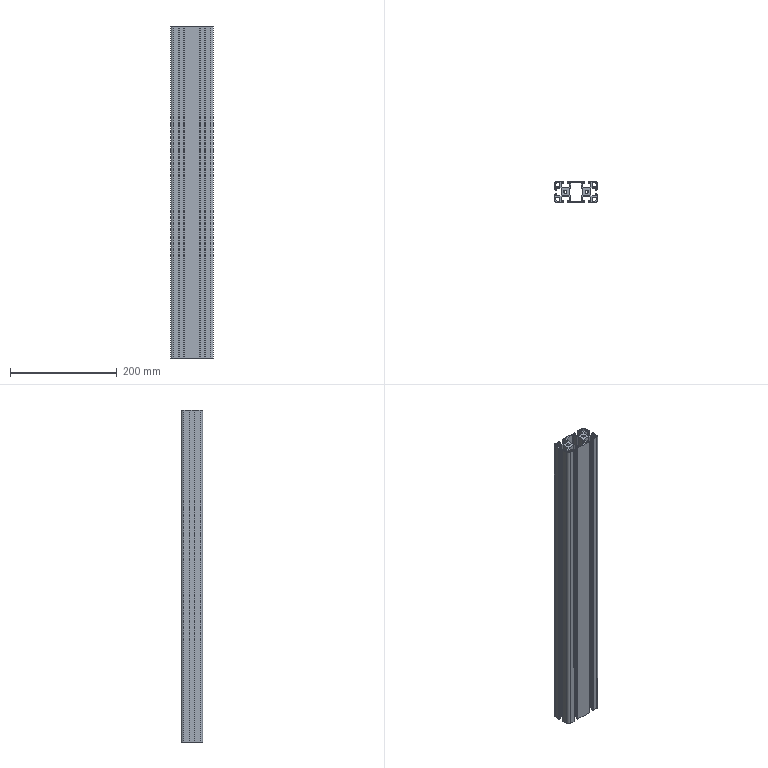Part | SolidWorks | features Fillet 2, Extrusion 1, ICE 1 | 1 solid | 170 faces | box 80 x 40 x 622 mm | volume 667832 mm3 | plane 142 | cylinder 28 | commonest cylinder face diameters 2 x16 10 x8 6 x4